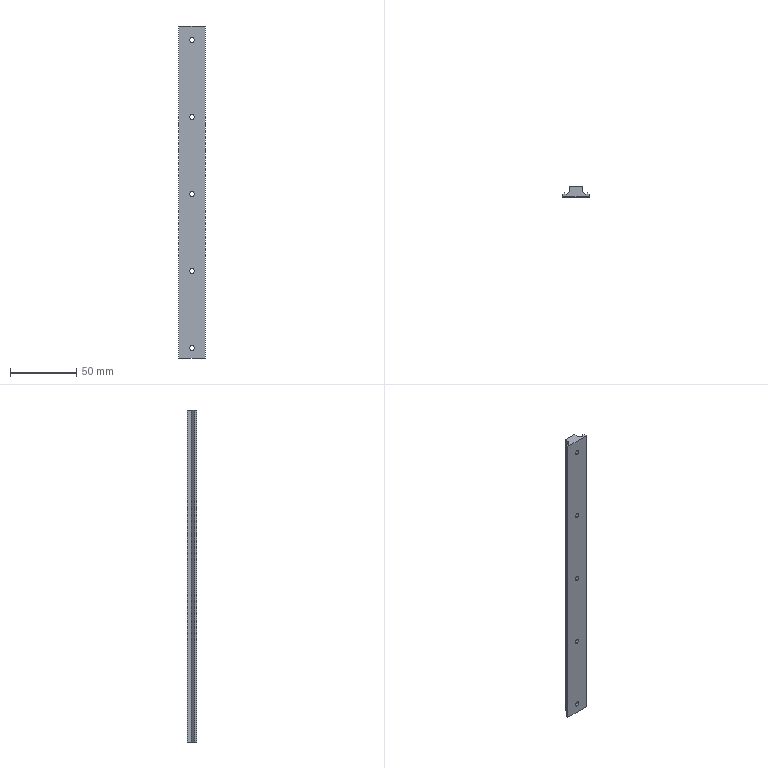Part | STEP file | Guide wheel mechanism revised.sldasm-Part-501 | 1 solid | 41 faces | box 20 x 7.5 x 250 mm | volume 23678 mm3 | plane 21 | cylinder 20 | commonest cylinder face diameters 3.5 x10 6 x10
STEP:
#1=CARTESIAN_POINT('',(0.,0.,237.75));
#2=VERTEX_POINT('',#1);
#3=CARTESIAN_POINT('',(0.,0.,241.25));
#4=VERTEX_POINT('',#3);
#5=CARTESIAN_POINT('',(0.,0.,239.5));
#6=DIRECTION('',(0.,1.,0.));
#7=DIRECTION('',(0.,0.,1.));
#8=AXIS2_PLACEMENT_3D('',#5,#6,#7);
#9=CIRCLE('',#8,1.75);
#10=EDGE_CURVE('',#2,#4,#9,.T.);
#11=ORIENTED_EDGE('',*,*,#10,.F.);
#12=CARTESIAN_POINT('',(0.,3.5,237.75));
#13=VERTEX_POINT('',#12);
#14=CARTESIAN_POINT('',(0.,0.,237.75));
#15=DIRECTION('',(0.,1.,0.));
#16=VECTOR('',#15,1000.);
#17=LINE('',#14,#16);
#18=EDGE_CURVE('',#2,#13,#17,.T.);
#19=ORIENTED_EDGE('',*,*,#18,.T.);
#20=CARTESIAN_POINT('',(0.,3.5,241.25));
#21=VERTEX_POINT('',#20);
#22=CARTESIAN_POINT('',(0.,3.5,239.5));
#23=DIRECTION('',(0.,1.,0.));
#24=DIRECTION('',(0.,0.,1.));
#25=AXIS2_PLACEMENT_3D('',#22,#23,#24);
#26=CIRCLE('',#25,1.75);
#27=EDGE_CURVE('',#13,#21,#26,.T.);
#28=ORIENTED_EDGE('',*,*,#27,.T.);
#29=CARTESIAN_POINT('',(0.,0.,241.25));
#30=DIRECTION('',(0.,1.,0.));
#31=VECTOR('',#30,1000.);
#32=LINE('',#29,#31);
#33=EDGE_CURVE('',#4,#21,#32,.T.);
#34=ORIENTED_EDGE('',*,*,#33,.F.);
#35=EDGE_LOOP('',(#11,#19,#28,#34));
#36=FACE_OUTER_BOUND('',#35,.T.);
#37=CARTESIAN_POINT('',(0.,0.,239.5));
#38=DIRECTION('',(0.,1.,0.));
#39=DIRECTION('',(0.,0.,1.));
#40=AXIS2_PLACEMENT_3D('',#37,#38,#39);
#41=CYLINDRICAL_SURFACE('',#40,1.75);
#42=ADVANCED_FACE('',(#36),#41,.F.);
#43=CARTESIAN_POINT('',(0.,3.5,236.5));
#44=VERTEX_POINT('',#43);
#45=CARTESIAN_POINT('',(0.,3.5,242.5));
#46=VERTEX_POINT('',#45);
#47=CARTESIAN_POINT('',(0.,3.5,239.5));
#48=DIRECTION('',(0.,1.,0.));
#49=DIRECTION('',(0.,0.,1.));
#50=AXIS2_PLACEMENT_3D('',#47,#48,#49);
#51=CIRCLE('',#50,3.);
#52=EDGE_CURVE('',#44,#46,#51,.T.);
#53=ORIENTED_EDGE('',*,*,#52,.F.);
#54=CARTESIAN_POINT('',(0.,7.5,236.5));
#55=VERTEX_POINT('',#54);
#56=CARTESIAN_POINT('',(0.,0.,236.5));
#57=DIRECTION('',(0.,1.,0.));
#58=VECTOR('',#57,1000.);
#59=LINE('',#56,#58);
#60=EDGE_CURVE('',#44,#55,#59,.T.);
#61=ORIENTED_EDGE('',*,*,#60,.T.);
#62=CARTESIAN_POINT('',(0.,7.5,242.5));
#63=VERTEX_POINT('',#62);
#64=CARTESIAN_POINT('',(0.,7.5,239.5));
#65=DIRECTION('',(0.,1.,0.));
#66=DIRECTION('',(0.,0.,1.));
#67=AXIS2_PLACEMENT_3D('',#64,#65,#66);
#68=CIRCLE('',#67,3.);
#69=EDGE_CURVE('',#55,#63,#68,.T.);
#70=ORIENTED_EDGE('',*,*,#69,.T.);
#71=CARTESIAN_POINT('',(0.,0.,242.5));
#72=DIRECTION('',(0.,1.,0.));
#73=VECTOR('',#72,1000.);
#74=LINE('',#71,#73);
#75=EDGE_CURVE('',#46,#63,#74,.T.);
#76=ORIENTED_EDGE('',*,*,#75,.F.);
#77=EDGE_LOOP('',(#53,#61,#70,#76));
#78=FACE_OUTER_BOUND('',#77,.T.);
#79=CARTESIAN_POINT('',(0.,0.,239.5));
#80=DIRECTION('',(0.,1.,0.));
#81=DIRECTION('',(0.,0.,1.));
#82=AXIS2_PLACEMENT_3D('',#79,#80,#81);
#83=CYLINDRICAL_SURFACE('',#82,3.);
#84=ADVANCED_FACE('',(#78),#83,.F.);
#85=CARTESIAN_POINT('',(0.,0.,179.75));
#86=VERTEX_POINT('',#85);
#87=CARTESIAN_POINT('',(0.,0.,183.25));
#88=VERTEX_POINT('',#87);
#89=CARTESIAN_POINT('',(0.,0.,181.5));
#90=DIRECTION('',(0.,1.,0.));
#91=DIRECTION('',(0.,0.,1.));
#92=AXIS2_PLACEMENT_3D('',#89,#90,#91);
#93=CIRCLE('',#92,1.75);
#94=EDGE_CURVE('',#86,#88,#93,.T.);
#95=ORIENTED_EDGE('',*,*,#94,.F.);
#96=CARTESIAN_POINT('',(0.,3.5,179.75));
#97=VERTEX_POINT('',#96);
#98=CARTESIAN_POINT('',(0.,0.,179.75));
#99=DIRECTION('',(0.,1.,0.));
#100=VECTOR('',#99,1000.);
#101=LINE('',#98,#100);
#102=EDGE_CURVE('',#86,#97,#101,.T.);
#103=ORIENTED_EDGE('',*,*,#102,.T.);
#104=CARTESIAN_POINT('',(0.,3.5,183.25));
#105=VERTEX_POINT('',#104);
#106=CARTESIAN_POINT('',(0.,3.5,181.5));
#107=DIRECTION('',(0.,1.,0.));
#108=DIRECTION('',(0.,0.,1.));
#109=AXIS2_PLACEMENT_3D('',#106,#107,#108);
#110=CIRCLE('',#109,1.75);
#111=EDGE_CURVE('',#97,#105,#110,.T.);
#112=ORIENTED_EDGE('',*,*,#111,.T.);
#113=CARTESIAN_POINT('',(0.,0.,183.25));
#114=DIRECTION('',(0.,1.,0.));
#115=VECTOR('',#114,1000.);
#116=LINE('',#113,#115);
#117=EDGE_CURVE('',#88,#105,#116,.T.);
#118=ORIENTED_EDGE('',*,*,#117,.F.);
#119=EDGE_LOOP('',(#95,#103,#112,#118));
#120=FACE_OUTER_BOUND('',#119,.T.);
#121=CARTESIAN_POINT('',(0.,0.,181.5));
#122=DIRECTION('',(0.,1.,0.));
#123=DIRECTION('',(0.,0.,1.));
#124=AXIS2_PLACEMENT_3D('',#121,#122,#123);
#125=CYLINDRICAL_SURFACE('',#124,1.75);
#126=ADVANCED_FACE('',(#120),#125,.F.);
#127=CARTESIAN_POINT('',(0.,3.5,178.5));
#128=VERTEX_POINT('',#127);
#129=CARTESIAN_POINT('',(0.,3.5,184.5));
#130=VERTEX_POINT('',#129);
#131=CARTESIAN_POINT('',(0.,3.5,181.5));
#132=DIRECTION('',(0.,1.,0.));
#133=DIRECTION('',(0.,0.,1.));
#134=AXIS2_PLACEMENT_3D('',#131,#132,#133);
#135=CIRCLE('',#134,3.);
#136=EDGE_CURVE('',#128,#130,#135,.T.);
#137=ORIENTED_EDGE('',*,*,#136,.F.);
#138=CARTESIAN_POINT('',(0.,7.5,178.5));
#139=VERTEX_POINT('',#138);
#140=CARTESIAN_POINT('',(0.,0.,178.5));
#141=DIRECTION('',(0.,1.,0.));
#142=VECTOR('',#141,1000.);
#143=LINE('',#140,#142);
#144=EDGE_CURVE('',#128,#139,#143,.T.);
#145=ORIENTED_EDGE('',*,*,#144,.T.);
#146=CARTESIAN_POINT('',(0.,7.5,184.5));
#147=VERTEX_POINT('',#146);
#148=CARTESIAN_POINT('',(0.,7.5,181.5));
#149=DIRECTION('',(0.,1.,0.));
#150=DIRECTION('',(0.,0.,1.));
#151=AXIS2_PLACEMENT_3D('',#148,#149,#150);
#152=CIRCLE('',#151,3.);
#153=EDGE_CURVE('',#139,#147,#152,.T.);
#154=ORIENTED_EDGE('',*,*,#153,.T.);
#155=CARTESIAN_POINT('',(0.,0.,184.5));
#156=DIRECTION('',(0.,1.,0.));
#157=VECTOR('',#156,1000.);
#158=LINE('',#155,#157);
#159=EDGE_CURVE('',#130,#147,#158,.T.);
#160=ORIENTED_EDGE('',*,*,#159,.F.);
#161=EDGE_LOOP('',(#137,#145,#154,#160));
#162=FACE_OUTER_BOUND('',#161,.T.);
#163=CARTESIAN_POINT('',(0.,0.,181.5));
#164=DIRECTION('',(0.,1.,0.));
#165=DIRECTION('',(0.,0.,1.));
#166=AXIS2_PLACEMENT_3D('',#163,#164,#165);
#167=CYLINDRICAL_SURFACE('',#166,3.);
#168=ADVANCED_FACE('',(#162),#167,.F.);
#169=CARTESIAN_POINT('',(0.,0.,121.75));
#170=VERTEX_POINT('',#169);
#171=CARTESIAN_POINT('',(0.,0.,125.25));
#172=VERTEX_POINT('',#171);
#173=CARTESIAN_POINT('',(0.,0.,123.5));
#174=DIRECTION('',(0.,1.,0.));
#175=DIRECTION('',(0.,0.,1.));
#176=AXIS2_PLACEMENT_3D('',#173,#174,#175);
#177=CIRCLE('',#176,1.75);
#178=EDGE_CURVE('',#170,#172,#177,.T.);
#179=ORIENTED_EDGE('',*,*,#178,.F.);
#180=CARTESIAN_POINT('',(0.,3.5,121.75));
#181=VERTEX_POINT('',#180);
#182=CARTESIAN_POINT('',(0.,0.,121.75));
#183=DIRECTION('',(0.,1.,0.));
#184=VECTOR('',#183,1000.);
#185=LINE('',#182,#184);
#186=EDGE_CURVE('',#170,#181,#185,.T.);
#187=ORIENTED_EDGE('',*,*,#186,.T.);
#188=CARTESIAN_POINT('',(0.,3.5,125.25));
#189=VERTEX_POINT('',#188);
#190=CARTESIAN_POINT('',(0.,3.5,123.5));
#191=DIRECTION('',(0.,1.,0.));
#192=DIRECTION('',(0.,0.,1.));
#193=AXIS2_PLACEMENT_3D('',#190,#191,#192);
#194=CIRCLE('',#193,1.75);
#195=EDGE_CURVE('',#181,#189,#194,.T.);
#196=ORIENTED_EDGE('',*,*,#195,.T.);
#197=CARTESIAN_POINT('',(0.,0.,125.25));
#198=DIRECTION('',(0.,1.,0.));
#199=VECTOR('',#198,1000.);
#200=LINE('',#197,#199);
#201=EDGE_CURVE('',#172,#189,#200,.T.);
#202=ORIENTED_EDGE('',*,*,#201,.F.);
#203=EDGE_LOOP('',(#179,#187,#196,#202));
#204=FACE_OUTER_BOUND('',#203,.T.);
#205=CARTESIAN_POINT('',(0.,0.,123.5));
#206=DIRECTION('',(0.,1.,0.));
#207=DIRECTION('',(0.,0.,1.));
#208=AXIS2_PLACEMENT_3D('',#205,#206,#207);
#209=CYLINDRICAL_SURFACE('',#208,1.75);
#210=ADVANCED_FACE('',(#204),#209,.F.);
#211=CARTESIAN_POINT('',(0.,3.5,120.5));
#212=VERTEX_POINT('',#211);
#213=CARTESIAN_POINT('',(0.,3.5,126.5));
#214=VERTEX_POINT('',#213);
#215=CARTESIAN_POINT('',(0.,3.5,123.5));
#216=DIRECTION('',(0.,1.,0.));
#217=DIRECTION('',(0.,0.,1.));
#218=AXIS2_PLACEMENT_3D('',#215,#216,#217);
#219=CIRCLE('',#218,3.);
#220=EDGE_CURVE('',#212,#214,#219,.T.);
#221=ORIENTED_EDGE('',*,*,#220,.F.);
#222=CARTESIAN_POINT('',(0.,7.5,120.5));
#223=VERTEX_POINT('',#222);
#224=CARTESIAN_POINT('',(0.,0.,120.5));
#225=DIRECTION('',(0.,1.,0.));
#226=VECTOR('',#225,1000.);
#227=LINE('',#224,#226);
#228=EDGE_CURVE('',#212,#223,#227,.T.);
#229=ORIENTED_EDGE('',*,*,#228,.T.);
#230=CARTESIAN_POINT('',(0.,7.5,126.5));
#231=VERTEX_POINT('',#230);
#232=CARTESIAN_POINT('',(0.,7.5,123.5));
#233=DIRECTION('',(0.,1.,0.));
#234=DIRECTION('',(0.,0.,1.));
#235=AXIS2_PLACEMENT_3D('',#232,#233,#234);
#236=CIRCLE('',#235,3.);
#237=EDGE_CURVE('',#223,#231,#236,.T.);
#238=ORIENTED_EDGE('',*,*,#237,.T.);
#239=CARTESIAN_POINT('',(0.,0.,126.5));
#240=DIRECTION('',(0.,1.,0.));
#241=VECTOR('',#240,1000.);
#242=LINE('',#239,#241);
#243=EDGE_CURVE('',#214,#231,#242,.T.);
#244=ORIENTED_EDGE('',*,*,#243,.F.);
#245=EDGE_LOOP('',(#221,#229,#238,#244));
#246=FACE_OUTER_BOUND('',#245,.T.);
#247=CARTESIAN_POINT('',(0.,0.,123.5));
#248=DIRECTION('',(0.,1.,0.));
#249=DIRECTION('',(0.,0.,1.));
#250=AXIS2_PLACEMENT_3D('',#247,#248,#249);
#251=CYLINDRICAL_SURFACE('',#250,3.);
#252=ADVANCED_FACE('',(#246),#251,.F.);
#253=CARTESIAN_POINT('',(0.,0.,63.75));
#254=VERTEX_POINT('',#253);
#255=CARTESIAN_POINT('',(0.,0.,67.25));
#256=VERTEX_POINT('',#255);
#257=CARTESIAN_POINT('',(0.,0.,65.5));
#258=DIRECTION('',(0.,1.,0.));
#259=DIRECTION('',(0.,0.,1.));
#260=AXIS2_PLACEMENT_3D('',#257,#258,#259);
#261=CIRCLE('',#260,1.75);
#262=EDGE_CURVE('',#254,#256,#261,.T.);
#263=ORIENTED_EDGE('',*,*,#262,.F.);
#264=CARTESIAN_POINT('',(0.,3.5,63.75));
#265=VERTEX_POINT('',#264);
#266=CARTESIAN_POINT('',(0.,0.,63.75));
#267=DIRECTION('',(0.,1.,0.));
#268=VECTOR('',#267,1000.);
#269=LINE('',#266,#268);
#270=EDGE_CURVE('',#254,#265,#269,.T.);
#271=ORIENTED_EDGE('',*,*,#270,.T.);
#272=CARTESIAN_POINT('',(0.,3.5,67.25));
#273=VERTEX_POINT('',#272);
#274=CARTESIAN_POINT('',(0.,3.5,65.5));
#275=DIRECTION('',(0.,1.,0.));
#276=DIRECTION('',(0.,0.,1.));
#277=AXIS2_PLACEMENT_3D('',#274,#275,#276);
#278=CIRCLE('',#277,1.75);
#279=EDGE_CURVE('',#265,#273,#278,.T.);
#280=ORIENTED_EDGE('',*,*,#279,.T.);
#281=CARTESIAN_POINT('',(0.,0.,67.25));
#282=DIRECTION('',(0.,1.,0.));
#283=VECTOR('',#282,1000.);
#284=LINE('',#281,#283);
#285=EDGE_CURVE('',#256,#273,#284,.T.);
#286=ORIENTED_EDGE('',*,*,#285,.F.);
#287=EDGE_LOOP('',(#263,#271,#280,#286));
#288=FACE_OUTER_BOUND('',#287,.T.);
#289=CARTESIAN_POINT('',(0.,0.,65.5));
#290=DIRECTION('',(0.,1.,0.));
#291=DIRECTION('',(0.,0.,1.));
#292=AXIS2_PLACEMENT_3D('',#289,#290,#291);
#293=CYLINDRICAL_SURFACE('',#292,1.75);
#294=ADVANCED_FACE('',(#288),#293,.F.);
#295=CARTESIAN_POINT('',(0.,3.5,62.5));
#296=VERTEX_POINT('',#295);
#297=CARTESIAN_POINT('',(0.,3.5,68.5));
#298=VERTEX_POINT('',#297);
#299=CARTESIAN_POINT('',(0.,3.5,65.5));
#300=DIRECTION('',(0.,1.,0.));
#301=DIRECTION('',(0.,0.,1.));
#302=AXIS2_PLACEMENT_3D('',#299,#300,#301);
#303=CIRCLE('',#302,3.);
#304=EDGE_CURVE('',#296,#298,#303,.T.);
#305=ORIENTED_EDGE('',*,*,#304,.F.);
#306=CARTESIAN_POINT('',(0.,7.5,62.5));
#307=VERTEX_POINT('',#306);
#308=CARTESIAN_POINT('',(0.,0.,62.5));
#309=DIRECTION('',(0.,1.,0.));
#310=VECTOR('',#309,1000.);
#311=LINE('',#308,#310);
#312=EDGE_CURVE('',#296,#307,#311,.T.);
#313=ORIENTED_EDGE('',*,*,#312,.T.);
#314=CARTESIAN_POINT('',(0.,7.5,68.5));
#315=VERTEX_POINT('',#314);
#316=CARTESIAN_POINT('',(0.,7.5,65.5));
#317=DIRECTION('',(0.,1.,0.));
#318=DIRECTION('',(0.,0.,1.));
#319=AXIS2_PLACEMENT_3D('',#316,#317,#318);
#320=CIRCLE('',#319,3.);
#321=EDGE_CURVE('',#307,#315,#320,.T.);
#322=ORIENTED_EDGE('',*,*,#321,.T.);
#323=CARTESIAN_POINT('',(0.,0.,68.5));
#324=DIRECTION('',(0.,1.,0.));
#325=VECTOR('',#324,1000.);
#326=LINE('',#323,#325);
#327=EDGE_CURVE('',#298,#315,#326,.T.);
#328=ORIENTED_EDGE('',*,*,#327,.F.);
#329=EDGE_LOOP('',(#305,#313,#322,#328));
#330=FACE_OUTER_BOUND('',#329,.T.);
#331=CARTESIAN_POINT('',(0.,0.,65.5));
#332=DIRECTION('',(0.,1.,0.));
#333=DIRECTION('',(0.,0.,1.));
#334=AXIS2_PLACEMENT_3D('',#331,#332,#333);
#335=CYLINDRICAL_SURFACE('',#334,3.);
#336=ADVANCED_FACE('',(#330),#335,.F.);
#337=CARTESIAN_POINT('',(0.,0.,5.75));
#338=VERTEX_POINT('',#337);
#339=CARTESIAN_POINT('',(0.,0.,9.25));
#340=VERTEX_POINT('',#339);
#341=CARTESIAN_POINT('',(0.,0.,7.5));
#342=DIRECTION('',(0.,1.,0.));
#343=DIRECTION('',(0.,0.,1.));
#344=AXIS2_PLACEMENT_3D('',#341,#342,#343);
#345=CIRCLE('',#344,1.75);
#346=EDGE_CURVE('',#338,#340,#345,.T.);
#347=ORIENTED_EDGE('',*,*,#346,.F.);
#348=CARTESIAN_POINT('',(0.,3.5,5.75));
#349=VERTEX_POINT('',#348);
#350=CARTESIAN_POINT('',(0.,0.,5.75));
#351=DIRECTION('',(0.,1.,0.));
#352=VECTOR('',#351,1000.);
#353=LINE('',#350,#352);
#354=EDGE_CURVE('',#338,#349,#353,.T.);
#355=ORIENTED_EDGE('',*,*,#354,.T.);
#356=CARTESIAN_POINT('',(0.,3.5,9.25));
#357=VERTEX_POINT('',#356);
#358=CARTESIAN_POINT('',(0.,3.5,7.5));
#359=DIRECTION('',(0.,1.,0.));
#360=DIRECTION('',(0.,0.,1.));
#361=AXIS2_PLACEMENT_3D('',#358,#359,#360);
#362=CIRCLE('',#361,1.75);
#363=EDGE_CURVE('',#349,#357,#362,.T.);
#364=ORIENTED_EDGE('',*,*,#363,.T.);
#365=CARTESIAN_POINT('',(0.,0.,9.25));
#366=DIRECTION('',(0.,1.,0.));
#367=VECTOR('',#366,1000.);
#368=LINE('',#365,#367);
#369=EDGE_CURVE('',#340,#357,#368,.T.);
#370=ORIENTED_EDGE('',*,*,#369,.F.);
#371=EDGE_LOOP('',(#347,#355,#364,#370));
#372=FACE_OUTER_BOUND('',#371,.T.);
#373=CARTESIAN_POINT('',(0.,0.,7.5));
#374=DIRECTION('',(0.,1.,0.));
#375=DIRECTION('',(0.,0.,1.));
#376=AXIS2_PLACEMENT_3D('',#373,#374,#375);
#377=CYLINDRICAL_SURFACE('',#376,1.75);
#378=ADVANCED_FACE('',(#372),#377,.F.);
#379=CARTESIAN_POINT('',(0.,3.5,4.5));
#380=VERTEX_POINT('',#379);
#381=CARTESIAN_POINT('',(0.,3.5,10.5));
#382=VERTEX_POINT('',#381);
#383=CARTESIAN_POINT('',(0.,3.5,7.5));
#384=DIRECTION('',(0.,1.,0.));
#385=DIRECTION('',(0.,0.,1.));
#386=AXIS2_PLACEMENT_3D('',#383,#384,#385);
#387=CIRCLE('',#386,3.);
#388=EDGE_CURVE('',#380,#382,#387,.T.);
#389=ORIENTED_EDGE('',*,*,#388,.F.);
#390=CARTESIAN_POINT('',(0.,7.5,4.5));
#391=VERTEX_POINT('',#390);
#392=CARTESIAN_POINT('',(0.,0.,4.5));
#393=DIRECTION('',(0.,1.,0.));
#394=VECTOR('',#393,1000.);
#395=LINE('',#392,#394);
#396=EDGE_CURVE('',#380,#391,#395,.T.);
#397=ORIENTED_EDGE('',*,*,#396,.T.);
#398=CARTESIAN_POINT('',(0.,7.5,10.5));
#399=VERTEX_POINT('',#398);
#400=CARTESIAN_POINT('',(0.,7.5,7.5));
#401=DIRECTION('',(0.,1.,0.));
#402=DIRECTION('',(0.,0.,1.));
#403=AXIS2_PLACEMENT_3D('',#400,#401,#402);
#404=CIRCLE('',#403,3.);
#405=EDGE_CURVE('',#391,#399,#404,.T.);
#406=ORIENTED_EDGE('',*,*,#405,.T.);
#407=CARTESIAN_POINT('',(0.,0.,10.5));
#408=DIRECTION('',(0.,1.,0.));
#409=VECTOR('',#408,1000.);
#410=LINE('',#407,#409);
#411=EDGE_CURVE('',#382,#399,#410,.T.);
#412=ORIENTED_EDGE('',*,*,#411,.F.);
#413=EDGE_LOOP('',(#389,#397,#406,#412));
#414=FACE_OUTER_BOUND('',#413,.T.);
#415=CARTESIAN_POINT('',(0.,0.,7.5));
#416=DIRECTION('',(0.,1.,0.));
#417=DIRECTION('',(0.,0.,1.));
#418=AXIS2_PLACEMENT_3D('',#415,#416,#417);
#419=CYLINDRICAL_SURFACE('',#418,3.);
#420=ADVANCED_FACE('',(#414),#419,.F.);
#421=CARTESIAN_POINT('',(0.,0.,181.5));
#422=DIRECTION('',(0.,1.,0.));
#423=DIRECTION('',(0.,0.,1.));
#424=AXIS2_PLACEMENT_3D('',#421,#422,#423);
#425=CIRCLE('',#424,1.75);
#426=EDGE_CURVE('',#88,#86,#425,.T.);
#427=ORIENTED_EDGE('',*,*,#426,.T.);
#428=ORIENTED_EDGE('',*,*,#94,.T.);
#429=EDGE_LOOP('',(#427,#428));
#430=FACE_BOUND('',#429,.T.);
#431=CARTESIAN_POINT('',(0.,0.,65.5));
#432=DIRECTION('',(0.,1.,0.));
#433=DIRECTION('',(0.,0.,1.));
#434=AXIS2_PLACEMENT_3D('',#431,#432,#433);
#435=CIRCLE('',#434,1.75);
#436=EDGE_CURVE('',#256,#254,#435,.T.);
#437=ORIENTED_EDGE('',*,*,#436,.T.);
#438=ORIENTED_EDGE('',*,*,#262,.T.);
#439=EDGE_LOOP('',(#437,#438));
#440=FACE_BOUND('',#439,.T.);
#441=CARTESIAN_POINT('',(-10.,0.,0.));
#442=VERTEX_POINT('',#441);
#443=CARTESIAN_POINT('',(10.,0.,0.));
#444=VERTEX_POINT('',#443);
#445=CARTESIAN_POINT('',(-10.,0.,0.));
#446=DIRECTION('',(1.,0.,0.));
#447=VECTOR('',#446,1000.);
#448=LINE('',#445,#447);
#449=EDGE_CURVE('',#442,#444,#448,.T.);
#450=ORIENTED_EDGE('',*,*,#449,.T.);
#451=CARTESIAN_POINT('',(10.,0.,250.));
#452=VERTEX_POINT('',#451);
#453=CARTESIAN_POINT('',(10.,0.,250.));
#454=DIRECTION('',(0.,0.,-1.));
#455=VECTOR('',#454,1000.);
#456=LINE('',#453,#455);
#457=EDGE_CURVE('',#452,#444,#456,.T.);
#458=ORIENTED_EDGE('',*,*,#457,.F.);
#459=CARTESIAN_POINT('',(-10.,0.,250.));
#460=VERTEX_POINT('',#459);
#461=CARTESIAN_POINT('',(-10.,0.,250.));
#462=DIRECTION('',(1.,0.,0.));
#463=VECTOR('',#462,1000.);
#464=LINE('',#461,#463);
#465=EDGE_CURVE('',#460,#452,#464,.T.);
#466=ORIENTED_EDGE('',*,*,#465,.F.);
#467=CARTESIAN_POINT('',(-10.,0.,250.));
#468=DIRECTION('',(0.,0.,-1.));
#469=VECTOR('',#468,1000.);
#470=LINE('',#467,#469);
#471=EDGE_CURVE('',#460,#442,#470,.T.);
#472=ORIENTED_EDGE('',*,*,#471,.T.);
#473=EDGE_LOOP('',(#450,#458,#466,#472));
#474=FACE_OUTER_BOUND('',#473,.T.);
#475=CARTESIAN_POINT('',(0.,0.,7.5));
#476=DIRECTION('',(0.,1.,0.));
#477=DIRECTION('',(0.,0.,1.));
#478=AXIS2_PLACEMENT_3D('',#475,#476,#477);
#479=CIRCLE('',#478,1.75);
#480=EDGE_CURVE('',#340,#338,#479,.T.);
#481=ORIENTED_EDGE('',*,*,#480,.T.);
#482=ORIENTED_EDGE('',*,*,#346,.T.);
#483=EDGE_LOOP('',(#481,#482));
#484=FACE_BOUND('',#483,.T.);
#485=CARTESIAN_POINT('',(0.,0.,123.5));
#486=DIRECTION('',(0.,1.,0.));
#487=DIRECTION('',(0.,0.,1.));
#488=AXIS2_PLACEMENT_3D('',#485,#486,#487);
#489=CIRCLE('',#488,1.75);
#490=EDGE_CURVE('',#172,#170,#489,.T.);
#491=ORIENTED_EDGE('',*,*,#490,.T.);
#492=ORIENTED_EDGE('',*,*,#178,.T.);
#493=EDGE_LOOP('',(#491,#492));
#494=FACE_BOUND('',#493,.T.);
#495=CARTESIAN_POINT('',(0.,0.,239.5));
#496=DIRECTION('',(0.,1.,0.));
#497=DIRECTION('',(0.,0.,1.));
#498=AXIS2_PLACEMENT_3D('',#495,#496,#497);
#499=CIRCLE('',#498,1.75);
#500=EDGE_CURVE('',#4,#2,#499,.T.);
#501=ORIENTED_EDGE('',*,*,#500,.T.);
#502=ORIENTED_EDGE('',*,*,#10,.T.);
#503=EDGE_LOOP('',(#501,#502));
#504=FACE_BOUND('',#503,.T.);
#505=CARTESIAN_POINT('',(-10.,0.,250.));
#506=DIRECTION('',(0.,1.,0.));
#507=DIRECTION('',(0.,0.,1.));
#508=AXIS2_PLACEMENT_3D('',#505,#506,#507);
#509=PLANE('',#508);
#510=ADVANCED_FACE('',(#430,#440,#474,#484,#494,#504),#509,.F.);
#511=CARTESIAN_POINT('',(0.,7.5,181.5));
#512=DIRECTION('',(0.,1.,0.));
#513=DIRECTION('',(0.,0.,1.));
#514=AXIS2_PLACEMENT_3D('',#511,#512,#513);
#515=CIRCLE('',#514,3.);
#516=EDGE_CURVE('',#147,#139,#515,.T.);
#517=ORIENTED_EDGE('',*,*,#516,.F.);
#518=ORIENTED_EDGE('',*,*,#153,.F.);
#519=EDGE_LOOP('',(#517,#518));
#520=FACE_BOUND('',#519,.T.);
#521=CARTESIAN_POINT('',(0.,7.5,65.5));
#522=DIRECTION('',(0.,1.,0.));
#523=DIRECTION('',(0.,0.,1.));
#524=AXIS2_PLACEMENT_3D('',#521,#522,#523);
#525=CIRCLE('',#524,3.);
#526=EDGE_CURVE('',#315,#307,#525,.T.);
#527=ORIENTED_EDGE('',*,*,#526,.F.);
#528=ORIENTED_EDGE('',*,*,#321,.F.);
#529=EDGE_LOOP('',(#527,#528));
#530=FACE_BOUND('',#529,.T.);
#531=CARTESIAN_POINT('',(4.864,7.5,0.));
#532=VERTEX_POINT('',#531);
#533=CARTESIAN_POINT('',(-4.864,7.5,0.));
#534=VERTEX_POINT('',#533);
#535=CARTESIAN_POINT('',(4.864,7.5,0.));
#536=DIRECTION('',(-1.,0.,0.));
#537=VECTOR('',#536,1000.);
#538=LINE('',#535,#537);
#539=EDGE_CURVE('',#532,#534,#538,.T.);
#540=ORIENTED_EDGE('',*,*,#539,.T.);
#541=CARTESIAN_POINT('',(-4.864,7.5,250.));
#542=VERTEX_POINT('',#541);
#543=CARTESIAN_POINT('',(-4.864,7.5,250.));
#544=DIRECTION('',(0.,0.,-1.));
#545=VECTOR('',#544,1000.);
#546=LINE('',#543,#545);
#547=EDGE_CURVE('',#542,#534,#546,.T.);
#548=ORIENTED_EDGE('',*,*,#547,.F.);
#549=CARTESIAN_POINT('',(4.864,7.5,250.));
#550=VERTEX_POINT('',#549);
#551=CARTESIAN_POINT('',(4.864,7.5,250.));
#552=DIRECTION('',(-1.,0.,0.));
#553=VECTOR('',#552,1000.);
#554=LINE('',#551,#553);
#555=EDGE_CURVE('',#550,#542,#554,.T.);
#556=ORIENTED_EDGE('',*,*,#555,.F.);
#557=CARTESIAN_POINT('',(4.864,7.5,250.));
#558=DIRECTION('',(0.,0.,-1.));
#559=VECTOR('',#558,1000.);
#560=LINE('',#557,#559);
#561=EDGE_CURVE('',#550,#532,#560,.T.);
#562=ORIENTED_EDGE('',*,*,#561,.T.);
#563=EDGE_LOOP('',(#540,#548,#556,#562));
#564=FACE_OUTER_BOUND('',#563,.T.);
#565=CARTESIAN_POINT('',(0.,7.5,7.5));
#566=DIRECTION('',(0.,1.,0.));
#567=DIRECTION('',(0.,0.,1.));
#568=AXIS2_PLACEMENT_3D('',#565,#566,#567);
#569=CIRCLE('',#568,3.);
#570=EDGE_CURVE('',#399,#391,#569,.T.);
#571=ORIENTED_EDGE('',*,*,#570,.F.);
#572=ORIENTED_EDGE('',*,*,#405,.F.);
#573=EDGE_LOOP('',(#571,#572));
#574=FACE_BOUND('',#573,.T.);
#575=CARTESIAN_POINT('',(0.,7.5,123.5));
#576=DIRECTION('',(0.,1.,0.));
#577=DIRECTION('',(0.,0.,1.));
#578=AXIS2_PLACEMENT_3D('',#575,#576,#577);
#579=CIRCLE('',#578,3.);
#580=EDGE_CURVE('',#231,#223,#579,.T.);
#581=ORIENTED_EDGE('',*,*,#580,.F.);
#582=ORIENTED_EDGE('',*,*,#237,.F.);
#583=EDGE_LOOP('',(#581,#582));
#584=FACE_BOUND('',#583,.T.);
#585=CARTESIAN_POINT('',(0.,7.5,239.5));
#586=DIRECTION('',(0.,1.,0.));
#587=DIRECTION('',(0.,0.,1.));
#588=AXIS2_PLACEMENT_3D('',#585,#586,#587);
#589=CIRCLE('',#588,3.);
#590=EDGE_CURVE('',#63,#55,#589,.T.);
#591=ORIENTED_EDGE('',*,*,#590,.F.);
#592=ORIENTED_EDGE('',*,*,#69,.F.);
#593=EDGE_LOOP('',(#591,#592));
#594=FACE_BOUND('',#593,.T.);
#595=CARTESIAN_POINT('',(4.864,7.5,250.));
#596=DIRECTION('',(0.,-1.,0.));
#597=DIRECTION('',(0.,0.,-1.));
#598=AXIS2_PLACEMENT_3D('',#595,#596,#597);
#599=PLANE('',#598);
#600=ADVANCED_FACE('',(#520,#530,#564,#574,#584,#594),#599,.F.);
#601=CARTESIAN_POINT('',(-10.,1.8,0.));
#602=VERTEX_POINT('',#601);
#603=CARTESIAN_POINT('',(-10.,1.8,0.));
#604=DIRECTION('',(0.,-1.,0.));
#605=VECTOR('',#604,1000.);
#606=LINE('',#603,#605);
#607=EDGE_CURVE('',#602,#442,#606,.T.);
#608=ORIENTED_EDGE('',*,*,#607,.T.);
#609=ORIENTED_EDGE('',*,*,#471,.F.);
#610=CARTESIAN_POINT('',(-10.,1.8,250.));
#611=VERTEX_POINT('',#610);
#612=CARTESIAN_POINT('',(-10.,1.8,250.));
#613=DIRECTION('',(0.,-1.,0.));
#614=VECTOR('',#613,1000.);
#615=LINE('',#612,#614);
#616=EDGE_CURVE('',#611,#460,#615,.T.);
#617=ORIENTED_EDGE('',*,*,#616,.F.);
#618=CARTESIAN_POINT('',(-10.,1.8,250.));
#619=DIRECTION('',(0.,0.,-1.));
#620=VECTOR('',#619,1000.);
#621=LINE('',#618,#620);
#622=EDGE_CURVE('',#611,#602,#621,.T.);
#623=ORIENTED_EDGE('',*,*,#622,.T.);
#624=EDGE_LOOP('',(#608,#609,#617,#623));
#625=FACE_OUTER_BOUND('',#624,.T.);
#626=CARTESIAN_POINT('',(-10.,1.8,250.));
#627=DIRECTION('',(1.,0.,0.));
#628=DIRECTION('',(0.,0.,-1.));
#629=AXIS2_PLACEMENT_3D('',#626,#627,#628);
#630=PLANE('',#629);
#631=ADVANCED_FACE('',(#625),#630,.F.);
#632=CARTESIAN_POINT('',(10.,1.8,0.));
#633=VERTEX_POINT('',#632);
#634=CARTESIAN_POINT('',(10.,0.,0.));
#635=DIRECTION('',(0.,1.,0.));
#636=VECTOR('',#635,1000.);
#637=LINE('',#634,#636);
#638=EDGE_CURVE('',#444,#633,#637,.T.);
#639=ORIENTED_EDGE('',*,*,#638,.T.);
#640=CARTESIAN_POINT('',(10.,1.8,250.));
#641=VERTEX_POINT('',#640);
#642=CARTESIAN_POINT('',(10.,1.8,250.));
#643=DIRECTION('',(0.,0.,-1.));
#644=VECTOR('',#643,1000.);
#645=LINE('',#642,#644);
#646=EDGE_CURVE('',#641,#633,#645,.T.);
#647=ORIENTED_EDGE('',*,*,#646,.F.);
#648=CARTESIAN_POINT('',(10.,0.,250.));
#649=DIRECTION('',(0.,1.,0.));
#650=VECTOR('',#649,1000.);
#651=LINE('',#648,#650);
#652=EDGE_CURVE('',#452,#641,#651,.T.);
#653=ORIENTED_EDGE('',*,*,#652,.F.);
#654=ORIENTED_EDGE('',*,*,#457,.T.);
#655=EDGE_LOOP('',(#639,#647,#653,#654));
#656=FACE_OUTER_BOUND('',#655,.T.);
#657=CARTESIAN_POINT('',(10.,0.,250.));
#658=DIRECTION('',(-1.,0.,0.));
#659=DIRECTION('',(0.,0.,1.));
#660=AXIS2_PLACEMENT_3D('',#657,#658,#659);
#661=PLANE('',#660);
#662=ADVANCED_FACE('',(#656),#661,.F.);
#663=CARTESIAN_POINT('',(8.993,2.807,0.));
#664=VERTEX_POINT('',#663);
#665=CARTESIAN_POINT('',(10.,1.8,0.));
#666=DIRECTION('',(-0.7071,0.7071,0.));
#667=VECTOR('',#666,1000.);
#668=LINE('',#665,#667);
#669=EDGE_CURVE('',#633,#664,#668,.T.);
#670=ORIENTED_EDGE('',*,*,#669,.T.);
#671=CARTESIAN_POINT('',(8.993,2.807,250.));
#672=VERTEX_POINT('',#671);
#673=CARTESIAN_POINT('',(8.993,2.807,250.));
#674=DIRECTION('',(0.,0.,-1.));
#675=VECTOR('',#674,1000.);
#676=LINE('',#673,#675);
#677=EDGE_CURVE('',#672,#664,#676,.T.);
#678=ORIENTED_EDGE('',*,*,#677,.F.);
#679=CARTESIAN_POINT('',(10.,1.8,250.));
#680=DIRECTION('',(-0.7071,0.7071,0.));
#681=VECTOR('',#680,1000.);
#682=LINE('',#679,#681);
#683=EDGE_CURVE('',#641,#672,#682,.T.);
#684=ORIENTED_EDGE('',*,*,#683,.F.);
#685=ORIENTED_EDGE('',*,*,#646,.T.);
#686=EDGE_LOOP('',(#670,#678,#684,#685));
#687=FACE_OUTER_BOUND('',#686,.T.);
#688=CARTESIAN_POINT('',(10.,1.8,250.));
#689=DIRECTION('',(-0.7071,-0.7071,0.));
#690=DIRECTION('',(0.7071,-0.7071,0.));
#691=AXIS2_PLACEMENT_3D('',#688,#689,#690);
#692=PLANE('',#691);
#693=ADVANCED_FACE('',(#687),#692,.F.);
#694=CARTESIAN_POINT('',(7.508,1.322,0.));
#695=VERTEX_POINT('',#694);
#696=CARTESIAN_POINT('',(8.993,2.807,0.));
#697=DIRECTION('',(-0.7071,-0.7071,0.));
#698=VECTOR('',#697,1000.);
#699=LINE('',#696,#698);
#700=EDGE_CURVE('',#664,#695,#699,.T.);
#701=ORIENTED_EDGE('',*,*,#700,.T.);
#702=CARTESIAN_POINT('',(7.508,1.322,250.));
#703=VERTEX_POINT('',#702);
#704=CARTESIAN_POINT('',(7.508,1.322,250.));
#705=DIRECTION('',(0.,0.,-1.));
#706=VECTOR('',#705,1000.);
#707=LINE('',#704,#706);
#708=EDGE_CURVE('',#703,#695,#707,.T.);
#709=ORIENTED_EDGE('',*,*,#708,.F.);
#710=CARTESIAN_POINT('',(8.993,2.807,250.));
#711=DIRECTION('',(-0.7071,-0.7071,0.));
#712=VECTOR('',#711,1000.);
#713=LINE('',#710,#712);
#714=EDGE_CURVE('',#672,#703,#713,.T.);
#715=ORIENTED_EDGE('',*,*,#714,.F.);
#716=ORIENTED_EDGE('',*,*,#677,.T.);
#717=EDGE_LOOP('',(#701,#709,#715,#716));
#718=FACE_OUTER_BOUND('',#717,.T.);
#719=CARTESIAN_POINT('',(8.993,2.807,250.));
#720=DIRECTION('',(0.7071,-0.7071,0.));
#721=DIRECTION('',(0.7071,0.7071,0.));
#722=AXIS2_PLACEMENT_3D('',#719,#720,#721);
#723=PLANE('',#722);
#724=ADVANCED_FACE('',(#718),#723,.F.);
#725=CARTESIAN_POINT('',(4.68,4.151,0.));
#726=VERTEX_POINT('',#725);
#727=CARTESIAN_POINT('',(7.508,1.322,0.));
#728=DIRECTION('',(-0.7071,0.7071,0.));
#729=VECTOR('',#728,1000.);
#730=LINE('',#727,#729);
#731=EDGE_CURVE('',#695,#726,#730,.T.);
#732=ORIENTED_EDGE('',*,*,#731,.T.);
#733=CARTESIAN_POINT('',(4.68,4.151,250.));
#734=VERTEX_POINT('',#733);
#735=CARTESIAN_POINT('',(4.68,4.151,250.));
#736=DIRECTION('',(0.,0.,-1.));
#737=VECTOR('',#736,1000.);
#738=LINE('',#735,#737);
#739=EDGE_CURVE('',#734,#726,#738,.T.);
#740=ORIENTED_EDGE('',*,*,#739,.F.);
#741=CARTESIAN_POINT('',(7.508,1.322,250.));
#742=DIRECTION('',(-0.7071,0.7071,0.));
#743=VECTOR('',#742,1000.);
#744=LINE('',#741,#743);
#745=EDGE_CURVE('',#703,#734,#744,.T.);
#746=ORIENTED_EDGE('',*,*,#745,.F.);
#747=ORIENTED_EDGE('',*,*,#708,.T.);
#748=EDGE_LOOP('',(#732,#740,#746,#747));
#749=FACE_OUTER_BOUND('',#748,.T.);
#750=CARTESIAN_POINT('',(7.508,1.322,250.));
#751=DIRECTION('',(-0.7071,-0.7071,0.));
#752=DIRECTION('',(0.7071,-0.7071,0.));
#753=AXIS2_PLACEMENT_3D('',#750,#751,#752);
#754=PLANE('',#753);
#755=ADVANCED_FACE('',(#749),#754,.F.);
#756=CARTESIAN_POINT('',(4.864,4.336,0.));
#757=VERTEX_POINT('',#756);
#758=CARTESIAN_POINT('',(4.68,4.151,0.));
#759=DIRECTION('',(0.7071,0.7071,0.));
#760=VECTOR('',#759,1000.);
#761=LINE('',#758,#760);
#762=EDGE_CURVE('',#726,#757,#761,.T.);
#763=ORIENTED_EDGE('',*,*,#762,.T.);
#764=CARTESIAN_POINT('',(4.864,4.336,250.));
#765=VERTEX_POINT('',#764);
#766=CARTESIAN_POINT('',(4.864,4.336,250.));
#767=DIRECTION('',(0.,0.,-1.));
#768=VECTOR('',#767,1000.);
#769=LINE('',#766,#768);
#770=EDGE_CURVE('',#765,#757,#769,.T.);
#771=ORIENTED_EDGE('',*,*,#770,.F.);
#772=CARTESIAN_POINT('',(4.68,4.151,250.));
#773=DIRECTION('',(0.7071,0.7071,0.));
#774=VECTOR('',#773,1000.);
#775=LINE('',#772,#774);
#776=EDGE_CURVE('',#734,#765,#775,.T.);
#777=ORIENTED_EDGE('',*,*,#776,.F.);
#778=ORIENTED_EDGE('',*,*,#739,.T.);
#779=EDGE_LOOP('',(#763,#771,#777,#778));
#780=FACE_OUTER_BOUND('',#779,.T.);
#781=CARTESIAN_POINT('',(4.68,4.151,250.));
#782=DIRECTION('',(-0.7071,0.7071,0.));
#783=DIRECTION('',(-0.7071,-0.7071,0.));
#784=AXIS2_PLACEMENT_3D('',#781,#782,#783);
#785=PLANE('',#784);
#786=ADVANCED_FACE('',(#780),#785,.F.);
#787=CARTESIAN_POINT('',(4.864,4.336,0.));
#788=DIRECTION('',(0.,1.,0.));
#789=VECTOR('',#788,1000.);
#790=LINE('',#787,#789);
#791=EDGE_CURVE('',#757,#532,#790,.T.);
#792=ORIENTED_EDGE('',*,*,#791,.T.);
#793=ORIENTED_EDGE('',*,*,#561,.F.);
#794=CARTESIAN_POINT('',(4.864,4.336,250.));
#795=DIRECTION('',(0.,1.,0.));
#796=VECTOR('',#795,1000.);
#797=LINE('',#794,#796);
#798=EDGE_CURVE('',#765,#550,#797,.T.);
#799=ORIENTED_EDGE('',*,*,#798,.F.);
#800=ORIENTED_EDGE('',*,*,#770,.T.);
#801=EDGE_LOOP('',(#792,#793,#799,#800));
#802=FACE_OUTER_BOUND('',#801,.T.);
#803=CARTESIAN_POINT('',(4.864,4.336,250.));
#804=DIRECTION('',(-1.,0.,0.));
#805=DIRECTION('',(0.,0.,1.));
#806=AXIS2_PLACEMENT_3D('',#803,#804,#805);
#807=PLANE('',#806);
#808=ADVANCED_FACE('',(#802),#807,.F.);
#809=CARTESIAN_POINT('',(-4.864,4.336,0.));
#810=VERTEX_POINT('',#809);
#811=CARTESIAN_POINT('',(-4.864,7.5,0.));
#812=DIRECTION('',(0.,-1.,0.));
#813=VECTOR('',#812,1000.);
#814=LINE('',#811,#813);
#815=EDGE_CURVE('',#534,#810,#814,.T.);
#816=ORIENTED_EDGE('',*,*,#815,.T.);
#817=CARTESIAN_POINT('',(-4.864,4.336,250.));
#818=VERTEX_POINT('',#817);
#819=CARTESIAN_POINT('',(-4.864,4.336,250.));
#820=DIRECTION('',(0.,0.,-1.));
#821=VECTOR('',#820,1000.);
#822=LINE('',#819,#821);
#823=EDGE_CURVE('',#818,#810,#822,.T.);
#824=ORIENTED_EDGE('',*,*,#823,.F.);
#825=CARTESIAN_POINT('',(-4.864,7.5,250.));
#826=DIRECTION('',(0.,-1.,0.));
#827=VECTOR('',#826,1000.);
#828=LINE('',#825,#827);
#829=EDGE_CURVE('',#542,#818,#828,.T.);
#830=ORIENTED_EDGE('',*,*,#829,.F.);
#831=ORIENTED_EDGE('',*,*,#547,.T.);
#832=EDGE_LOOP('',(#816,#824,#830,#831));
#833=FACE_OUTER_BOUND('',#832,.T.);
#834=CARTESIAN_POINT('',(-4.864,7.5,250.));
#835=DIRECTION('',(1.,0.,0.));
#836=DIRECTION('',(0.,0.,-1.));
#837=AXIS2_PLACEMENT_3D('',#834,#835,#836);
#838=PLANE('',#837);
#839=ADVANCED_FACE('',(#833),#838,.F.);
#840=CARTESIAN_POINT('',(-4.68,4.151,0.));
#841=VERTEX_POINT('',#840);
#842=CARTESIAN_POINT('',(-4.864,4.336,0.));
#843=DIRECTION('',(0.7071,-0.7071,0.));
#844=VECTOR('',#843,1000.);
#845=LINE('',#842,#844);
#846=EDGE_CURVE('',#810,#841,#845,.T.);
#847=ORIENTED_EDGE('',*,*,#846,.T.);
#848=CARTESIAN_POINT('',(-4.68,4.151,250.));
#849=VERTEX_POINT('',#848);
#850=CARTESIAN_POINT('',(-4.68,4.151,250.));
#851=DIRECTION('',(0.,0.,-1.));
#852=VECTOR('',#851,1000.);
#853=LINE('',#850,#852);
#854=EDGE_CURVE('',#849,#841,#853,.T.);
#855=ORIENTED_EDGE('',*,*,#854,.F.);
#856=CARTESIAN_POINT('',(-4.864,4.336,250.));
#857=DIRECTION('',(0.7071,-0.7071,0.));
#858=VECTOR('',#857,1000.);
#859=LINE('',#856,#858);
#860=EDGE_CURVE('',#818,#849,#859,.T.);
#861=ORIENTED_EDGE('',*,*,#860,.F.);
#862=ORIENTED_EDGE('',*,*,#823,.T.);
#863=EDGE_LOOP('',(#847,#855,#861,#862));
#864=FACE_OUTER_BOUND('',#863,.T.);
#865=CARTESIAN_POINT('',(-4.864,4.336,250.));
#866=DIRECTION('',(0.7071,0.7071,0.));
#867=DIRECTION('',(-0.7071,0.7071,0.));
#868=AXIS2_PLACEMENT_3D('',#865,#866,#867);
#869=PLANE('',#868);
#870=ADVANCED_FACE('',(#864),#869,.F.);
#871=CARTESIAN_POINT('',(-7.508,1.322,0.));
#872=VERTEX_POINT('',#871);
#873=CARTESIAN_POINT('',(-4.68,4.151,0.));
#874=DIRECTION('',(-0.7071,-0.7071,0.));
#875=VECTOR('',#874,1000.);
#876=LINE('',#873,#875);
#877=EDGE_CURVE('',#841,#872,#876,.T.);
#878=ORIENTED_EDGE('',*,*,#877,.T.);
#879=CARTESIAN_POINT('',(-7.508,1.322,250.));
#880=VERTEX_POINT('',#879);
#881=CARTESIAN_POINT('',(-7.508,1.322,250.));
#882=DIRECTION('',(0.,0.,-1.));
#883=VECTOR('',#882,1000.);
#884=LINE('',#881,#883);
#885=EDGE_CURVE('',#880,#872,#884,.T.);
#886=ORIENTED_EDGE('',*,*,#885,.F.);
#887=CARTESIAN_POINT('',(-4.68,4.151,250.));
#888=DIRECTION('',(-0.7071,-0.7071,0.));
#889=VECTOR('',#888,1000.);
#890=LINE('',#887,#889);
#891=EDGE_CURVE('',#849,#880,#890,.T.);
#892=ORIENTED_EDGE('',*,*,#891,.F.);
#893=ORIENTED_EDGE('',*,*,#854,.T.);
#894=EDGE_LOOP('',(#878,#886,#892,#893));
#895=FACE_OUTER_BOUND('',#894,.T.);
#896=CARTESIAN_POINT('',(-4.68,4.151,250.));
#897=DIRECTION('',(0.7071,-0.7071,0.));
#898=DIRECTION('',(0.7071,0.7071,0.));
#899=AXIS2_PLACEMENT_3D('',#896,#897,#898);
#900=PLANE('',#899);
#901=ADVANCED_FACE('',(#895),#900,.F.);
#902=CARTESIAN_POINT('',(-8.993,2.807,0.));
#903=VERTEX_POINT('',#902);
#904=CARTESIAN_POINT('',(-7.508,1.322,0.));
#905=DIRECTION('',(-0.7071,0.7071,0.));
#906=VECTOR('',#905,1000.);
#907=LINE('',#904,#906);
#908=EDGE_CURVE('',#872,#903,#907,.T.);
#909=ORIENTED_EDGE('',*,*,#908,.T.);
#910=CARTESIAN_POINT('',(-8.993,2.807,250.));
#911=VERTEX_POINT('',#910);
#912=CARTESIAN_POINT('',(-8.993,2.807,250.));
#913=DIRECTION('',(0.,0.,-1.));
#914=VECTOR('',#913,1000.);
#915=LINE('',#912,#914);
#916=EDGE_CURVE('',#911,#903,#915,.T.);
#917=ORIENTED_EDGE('',*,*,#916,.F.);
#918=CARTESIAN_POINT('',(-7.508,1.322,250.));
#919=DIRECTION('',(-0.7071,0.7071,0.));
#920=VECTOR('',#919,1000.);
#921=LINE('',#918,#920);
#922=EDGE_CURVE('',#880,#911,#921,.T.);
#923=ORIENTED_EDGE('',*,*,#922,.F.);
#924=ORIENTED_EDGE('',*,*,#885,.T.);
#925=EDGE_LOOP('',(#909,#917,#923,#924));
#926=FACE_OUTER_BOUND('',#925,.T.);
#927=CARTESIAN_POINT('',(-7.508,1.322,250.));
#928=DIRECTION('',(-0.7071,-0.7071,0.));
#929=DIRECTION('',(0.7071,-0.7071,0.));
#930=AXIS2_PLACEMENT_3D('',#927,#928,#929);
#931=PLANE('',#930);
#932=ADVANCED_FACE('',(#926),#931,.F.);
#933=CARTESIAN_POINT('',(-8.993,2.807,0.));
#934=DIRECTION('',(-0.7071,-0.7071,0.));
#935=VECTOR('',#934,1000.);
#936=LINE('',#933,#935);
#937=EDGE_CURVE('',#903,#602,#936,.T.);
#938=ORIENTED_EDGE('',*,*,#937,.T.);
#939=ORIENTED_EDGE('',*,*,#622,.F.);
#940=CARTESIAN_POINT('',(-8.993,2.807,250.));
#941=DIRECTION('',(-0.7071,-0.7071,0.));
#942=VECTOR('',#941,1000.);
#943=LINE('',#940,#942);
#944=EDGE_CURVE('',#911,#611,#943,.T.);
#945=ORIENTED_EDGE('',*,*,#944,.F.);
#946=ORIENTED_EDGE('',*,*,#916,.T.);
#947=EDGE_LOOP('',(#938,#939,#945,#946));
#948=FACE_OUTER_BOUND('',#947,.T.);
#949=CARTESIAN_POINT('',(-8.993,2.807,250.));
#950=DIRECTION('',(0.7071,-0.7071,0.));
#951=DIRECTION('',(0.7071,0.7071,0.));
#952=AXIS2_PLACEMENT_3D('',#949,#950,#951);
#953=PLANE('',#952);
#954=ADVANCED_FACE('',(#948),#953,.F.);
#955=ORIENTED_EDGE('',*,*,#616,.T.);
#956=ORIENTED_EDGE('',*,*,#465,.T.);
#957=ORIENTED_EDGE('',*,*,#652,.T.);
#958=ORIENTED_EDGE('',*,*,#683,.T.);
#959=ORIENTED_EDGE('',*,*,#714,.T.);
#960=ORIENTED_EDGE('',*,*,#745,.T.);
#961=ORIENTED_EDGE('',*,*,#776,.T.);
#962=ORIENTED_EDGE('',*,*,#798,.T.);
#963=ORIENTED_EDGE('',*,*,#555,.T.);
#964=ORIENTED_EDGE('',*,*,#829,.T.);
#965=ORIENTED_EDGE('',*,*,#860,.T.);
#966=ORIENTED_EDGE('',*,*,#891,.T.);
#967=ORIENTED_EDGE('',*,*,#922,.T.);
#968=ORIENTED_EDGE('',*,*,#944,.T.);
#969=EDGE_LOOP('',(#955,#956,#957,#958,#959,#960,#961,#962,#963,#964,#965,#966,#967,#968));
#970=FACE_OUTER_BOUND('',#969,.T.);
#971=CARTESIAN_POINT('',(0.,0.,250.));
#972=DIRECTION('',(0.,0.,1.));
#973=DIRECTION('',(1.,0.,0.));
#974=AXIS2_PLACEMENT_3D('',#971,#972,#973);
#975=PLANE('',#974);
#976=ADVANCED_FACE('',(#970),#975,.T.);
#977=ORIENTED_EDGE('',*,*,#607,.F.);
#978=ORIENTED_EDGE('',*,*,#937,.F.);
#979=ORIENTED_EDGE('',*,*,#908,.F.);
#980=ORIENTED_EDGE('',*,*,#877,.F.);
#981=ORIENTED_EDGE('',*,*,#846,.F.);
#982=ORIENTED_EDGE('',*,*,#815,.F.);
#983=ORIENTED_EDGE('',*,*,#539,.F.);
#984=ORIENTED_EDGE('',*,*,#791,.F.);
#985=ORIENTED_EDGE('',*,*,#762,.F.);
#986=ORIENTED_EDGE('',*,*,#731,.F.);
#987=ORIENTED_EDGE('',*,*,#700,.F.);
#988=ORIENTED_EDGE('',*,*,#669,.F.);
#989=ORIENTED_EDGE('',*,*,#638,.F.);
#990=ORIENTED_EDGE('',*,*,#449,.F.);
#991=EDGE_LOOP('',(#977,#978,#979,#980,#981,#982,#983,#984,#985,#986,#987,#988,#989,#990));
#992=FACE_OUTER_BOUND('',#991,.T.);
#993=CARTESIAN_POINT('',(0.,0.,0.));
#994=DIRECTION('',(0.,0.,1.));
#995=DIRECTION('',(1.,0.,0.));
#996=AXIS2_PLACEMENT_3D('',#993,#994,#995);
#997=PLANE('',#996);
#998=ADVANCED_FACE('',(#992),#997,.F.);
#999=ORIENTED_EDGE('',*,*,#396,.F.);
#1000=CARTESIAN_POINT('',(0.,3.5,7.5));
#1001=DIRECTION('',(0.,1.,0.));
#1002=DIRECTION('',(0.,0.,1.));
#1003=AXIS2_PLACEMENT_3D('',#1000,#1001,#1002);
#1004=CIRCLE('',#1003,3.);
#1005=EDGE_CURVE('',#382,#380,#1004,.T.);
#1006=ORIENTED_EDGE('',*,*,#1005,.F.);
#1007=ORIENTED_EDGE('',*,*,#411,.T.);
#1008=ORIENTED_EDGE('',*,*,#570,.T.);
#1009=EDGE_LOOP('',(#999,#1006,#1007,#1008));
#1010=FACE_OUTER_BOUND('',#1009,.T.);
#1011=CARTESIAN_POINT('',(0.,0.,7.5));
#1012=DIRECTION('',(0.,1.,0.));
#1013=DIRECTION('',(0.,0.,1.));
#1014=AXIS2_PLACEMENT_3D('',#1011,#1012,#1013);
#1015=CYLINDRICAL_SURFACE('',#1014,3.);
#1016=ADVANCED_FACE('',(#1010),#1015,.F.);
#1017=ORIENTED_EDGE('',*,*,#1005,.T.);
#1018=ORIENTED_EDGE('',*,*,#388,.T.);
#1019=EDGE_LOOP('',(#1017,#1018));
#1020=FACE_OUTER_BOUND('',#1019,.T.);
#1021=CARTESIAN_POINT('',(0.,3.5,7.5));
#1022=DIRECTION('',(0.,1.,0.));
#1023=DIRECTION('',(0.,0.,1.));
#1024=AXIS2_PLACEMENT_3D('',#1021,#1022,#1023);
#1025=CIRCLE('',#1024,1.75);
#1026=EDGE_CURVE('',#357,#349,#1025,.T.);
#1027=ORIENTED_EDGE('',*,*,#1026,.F.);
#1028=ORIENTED_EDGE('',*,*,#363,.F.);
#1029=EDGE_LOOP('',(#1027,#1028));
#1030=FACE_BOUND('',#1029,.T.);
#1031=CARTESIAN_POINT('',(3.,3.5,7.5));
#1032=DIRECTION('',(0.,1.,0.));
#1033=DIRECTION('',(0.,0.,1.));
#1034=AXIS2_PLACEMENT_3D('',#1031,#1032,#1033);
#1035=PLANE('',#1034);
#1036=ADVANCED_FACE('',(#1020,#1030),#1035,.T.);
#1037=ORIENTED_EDGE('',*,*,#354,.F.);
#1038=ORIENTED_EDGE('',*,*,#480,.F.);
#1039=ORIENTED_EDGE('',*,*,#369,.T.);
#1040=ORIENTED_EDGE('',*,*,#1026,.T.);
#1041=EDGE_LOOP('',(#1037,#1038,#1039,#1040));
#1042=FACE_OUTER_BOUND('',#1041,.T.);
#1043=CARTESIAN_POINT('',(0.,0.,7.5));
#1044=DIRECTION('',(0.,1.,0.));
#1045=DIRECTION('',(0.,0.,1.));
#1046=AXIS2_PLACEMENT_3D('',#1043,#1044,#1045);
#1047=CYLINDRICAL_SURFACE('',#1046,1.75);
#1048=ADVANCED_FACE('',(#1042),#1047,.F.);
#1049=ORIENTED_EDGE('',*,*,#312,.F.);
#1050=CARTESIAN_POINT('',(0.,3.5,65.5));
#1051=DIRECTION('',(0.,1.,0.));
#1052=DIRECTION('',(0.,0.,1.));
#1053=AXIS2_PLACEMENT_3D('',#1050,#1051,#1052);
#1054=CIRCLE('',#1053,3.);
#1055=EDGE_CURVE('',#298,#296,#1054,.T.);
#1056=ORIENTED_EDGE('',*,*,#1055,.F.);
#1057=ORIENTED_EDGE('',*,*,#327,.T.);
#1058=ORIENTED_EDGE('',*,*,#526,.T.);
#1059=EDGE_LOOP('',(#1049,#1056,#1057,#1058));
#1060=FACE_OUTER_BOUND('',#1059,.T.);
#1061=CARTESIAN_POINT('',(0.,0.,65.5));
#1062=DIRECTION('',(0.,1.,0.));
#1063=DIRECTION('',(0.,0.,1.));
#1064=AXIS2_PLACEMENT_3D('',#1061,#1062,#1063);
#1065=CYLINDRICAL_SURFACE('',#1064,3.);
#1066=ADVANCED_FACE('',(#1060),#1065,.F.);
#1067=ORIENTED_EDGE('',*,*,#1055,.T.);
#1068=ORIENTED_EDGE('',*,*,#304,.T.);
#1069=EDGE_LOOP('',(#1067,#1068));
#1070=FACE_OUTER_BOUND('',#1069,.T.);
#1071=CARTESIAN_POINT('',(0.,3.5,65.5));
#1072=DIRECTION('',(0.,1.,0.));
#1073=DIRECTION('',(0.,0.,1.));
#1074=AXIS2_PLACEMENT_3D('',#1071,#1072,#1073);
#1075=CIRCLE('',#1074,1.75);
#1076=EDGE_CURVE('',#273,#265,#1075,.T.);
#1077=ORIENTED_EDGE('',*,*,#1076,.F.);
#1078=ORIENTED_EDGE('',*,*,#279,.F.);
#1079=EDGE_LOOP('',(#1077,#1078));
#1080=FACE_BOUND('',#1079,.T.);
#1081=CARTESIAN_POINT('',(3.,3.5,65.5));
#1082=DIRECTION('',(0.,1.,0.));
#1083=DIRECTION('',(0.,0.,1.));
#1084=AXIS2_PLACEMENT_3D('',#1081,#1082,#1083);
#1085=PLANE('',#1084);
#1086=ADVANCED_FACE('',(#1070,#1080),#1085,.T.);
#1087=ORIENTED_EDGE('',*,*,#270,.F.);
#1088=ORIENTED_EDGE('',*,*,#436,.F.);
#1089=ORIENTED_EDGE('',*,*,#285,.T.);
#1090=ORIENTED_EDGE('',*,*,#1076,.T.);
#1091=EDGE_LOOP('',(#1087,#1088,#1089,#1090));
#1092=FACE_OUTER_BOUND('',#1091,.T.);
#1093=CARTESIAN_POINT('',(0.,0.,65.5));
#1094=DIRECTION('',(0.,1.,0.));
#1095=DIRECTION('',(0.,0.,1.));
#1096=AXIS2_PLACEMENT_3D('',#1093,#1094,#1095);
#1097=CYLINDRICAL_SURFACE('',#1096,1.75);
#1098=ADVANCED_FACE('',(#1092),#1097,.F.);
#1099=ORIENTED_EDGE('',*,*,#228,.F.);
#1100=CARTESIAN_POINT('',(0.,3.5,123.5));
#1101=DIRECTION('',(0.,1.,0.));
#1102=DIRECTION('',(0.,0.,1.));
#1103=AXIS2_PLACEMENT_3D('',#1100,#1101,#1102);
#1104=CIRCLE('',#1103,3.);
#1105=EDGE_CURVE('',#214,#212,#1104,.T.);
#1106=ORIENTED_EDGE('',*,*,#1105,.F.);
#1107=ORIENTED_EDGE('',*,*,#243,.T.);
#1108=ORIENTED_EDGE('',*,*,#580,.T.);
#1109=EDGE_LOOP('',(#1099,#1106,#1107,#1108));
#1110=FACE_OUTER_BOUND('',#1109,.T.);
#1111=CARTESIAN_POINT('',(0.,0.,123.5));
#1112=DIRECTION('',(0.,1.,0.));
#1113=DIRECTION('',(0.,0.,1.));
#1114=AXIS2_PLACEMENT_3D('',#1111,#1112,#1113);
#1115=CYLINDRICAL_SURFACE('',#1114,3.);
#1116=ADVANCED_FACE('',(#1110),#1115,.F.);
#1117=ORIENTED_EDGE('',*,*,#1105,.T.);
#1118=ORIENTED_EDGE('',*,*,#220,.T.);
#1119=EDGE_LOOP('',(#1117,#1118));
#1120=FACE_OUTER_BOUND('',#1119,.T.);
#1121=CARTESIAN_POINT('',(0.,3.5,123.5));
#1122=DIRECTION('',(0.,1.,0.));
#1123=DIRECTION('',(0.,0.,1.));
#1124=AXIS2_PLACEMENT_3D('',#1121,#1122,#1123);
#1125=CIRCLE('',#1124,1.75);
#1126=EDGE_CURVE('',#189,#181,#1125,.T.);
#1127=ORIENTED_EDGE('',*,*,#1126,.F.);
#1128=ORIENTED_EDGE('',*,*,#195,.F.);
#1129=EDGE_LOOP('',(#1127,#1128));
#1130=FACE_BOUND('',#1129,.T.);
#1131=CARTESIAN_POINT('',(3.,3.5,123.5));
#1132=DIRECTION('',(0.,1.,0.));
#1133=DIRECTION('',(0.,0.,1.));
#1134=AXIS2_PLACEMENT_3D('',#1131,#1132,#1133);
#1135=PLANE('',#1134);
#1136=ADVANCED_FACE('',(#1120,#1130),#1135,.T.);
#1137=ORIENTED_EDGE('',*,*,#186,.F.);
#1138=ORIENTED_EDGE('',*,*,#490,.F.);
#1139=ORIENTED_EDGE('',*,*,#201,.T.);
#1140=ORIENTED_EDGE('',*,*,#1126,.T.);
#1141=EDGE_LOOP('',(#1137,#1138,#1139,#1140));
#1142=FACE_OUTER_BOUND('',#1141,.T.);
#1143=CARTESIAN_POINT('',(0.,0.,123.5));
#1144=DIRECTION('',(0.,1.,0.));
#1145=DIRECTION('',(0.,0.,1.));
#1146=AXIS2_PLACEMENT_3D('',#1143,#1144,#1145);
#1147=CYLINDRICAL_SURFACE('',#1146,1.75);
#1148=ADVANCED_FACE('',(#1142),#1147,.F.);
#1149=ORIENTED_EDGE('',*,*,#144,.F.);
#1150=CARTESIAN_POINT('',(0.,3.5,181.5));
#1151=DIRECTION('',(0.,1.,0.));
#1152=DIRECTION('',(0.,0.,1.));
#1153=AXIS2_PLACEMENT_3D('',#1150,#1151,#1152);
#1154=CIRCLE('',#1153,3.);
#1155=EDGE_CURVE('',#130,#128,#1154,.T.);
#1156=ORIENTED_EDGE('',*,*,#1155,.F.);
#1157=ORIENTED_EDGE('',*,*,#159,.T.);
#1158=ORIENTED_EDGE('',*,*,#516,.T.);
#1159=EDGE_LOOP('',(#1149,#1156,#1157,#1158));
#1160=FACE_OUTER_BOUND('',#1159,.T.);
#1161=CARTESIAN_POINT('',(0.,0.,181.5));
#1162=DIRECTION('',(0.,1.,0.));
#1163=DIRECTION('',(0.,0.,1.));
#1164=AXIS2_PLACEMENT_3D('',#1161,#1162,#1163);
#1165=CYLINDRICAL_SURFACE('',#1164,3.);
#1166=ADVANCED_FACE('',(#1160),#1165,.F.);
#1167=ORIENTED_EDGE('',*,*,#1155,.T.);
#1168=ORIENTED_EDGE('',*,*,#136,.T.);
#1169=EDGE_LOOP('',(#1167,#1168));
#1170=FACE_OUTER_BOUND('',#1169,.T.);
#1171=CARTESIAN_POINT('',(0.,3.5,181.5));
#1172=DIRECTION('',(0.,1.,0.));
#1173=DIRECTION('',(0.,0.,1.));
#1174=AXIS2_PLACEMENT_3D('',#1171,#1172,#1173);
#1175=CIRCLE('',#1174,1.75);
#1176=EDGE_CURVE('',#105,#97,#1175,.T.);
#1177=ORIENTED_EDGE('',*,*,#1176,.F.);
#1178=ORIENTED_EDGE('',*,*,#111,.F.);
#1179=EDGE_LOOP('',(#1177,#1178));
#1180=FACE_BOUND('',#1179,.T.);
#1181=CARTESIAN_POINT('',(3.,3.5,181.5));
#1182=DIRECTION('',(0.,1.,0.));
#1183=DIRECTION('',(0.,0.,1.));
#1184=AXIS2_PLACEMENT_3D('',#1181,#1182,#1183);
#1185=PLANE('',#1184);
#1186=ADVANCED_FACE('',(#1170,#1180),#1185,.T.);
#1187=ORIENTED_EDGE('',*,*,#102,.F.);
#1188=ORIENTED_EDGE('',*,*,#426,.F.);
#1189=ORIENTED_EDGE('',*,*,#117,.T.);
#1190=ORIENTED_EDGE('',*,*,#1176,.T.);
#1191=EDGE_LOOP('',(#1187,#1188,#1189,#1190));
#1192=FACE_OUTER_BOUND('',#1191,.T.);
#1193=CARTESIAN_POINT('',(0.,0.,181.5));
#1194=DIRECTION('',(0.,1.,0.));
#1195=DIRECTION('',(0.,0.,1.));
#1196=AXIS2_PLACEMENT_3D('',#1193,#1194,#1195);
#1197=CYLINDRICAL_SURFACE('',#1196,1.75);
#1198=ADVANCED_FACE('',(#1192),#1197,.F.);
#1199=ORIENTED_EDGE('',*,*,#60,.F.);
#1200=CARTESIAN_POINT('',(0.,3.5,239.5));
#1201=DIRECTION('',(0.,1.,0.));
#1202=DIRECTION('',(0.,0.,1.));
#1203=AXIS2_PLACEMENT_3D('',#1200,#1201,#1202);
#1204=CIRCLE('',#1203,3.);
#1205=EDGE_CURVE('',#46,#44,#1204,.T.);
#1206=ORIENTED_EDGE('',*,*,#1205,.F.);
#1207=ORIENTED_EDGE('',*,*,#75,.T.);
#1208=ORIENTED_EDGE('',*,*,#590,.T.);
#1209=EDGE_LOOP('',(#1199,#1206,#1207,#1208));
#1210=FACE_OUTER_BOUND('',#1209,.T.);
#1211=CARTESIAN_POINT('',(0.,0.,239.5));
#1212=DIRECTION('',(0.,1.,0.));
#1213=DIRECTION('',(0.,0.,1.));
#1214=AXIS2_PLACEMENT_3D('',#1211,#1212,#1213);
#1215=CYLINDRICAL_SURFACE('',#1214,3.);
#1216=ADVANCED_FACE('',(#1210),#1215,.F.);
#1217=ORIENTED_EDGE('',*,*,#1205,.T.);
#1218=ORIENTED_EDGE('',*,*,#52,.T.);
#1219=EDGE_LOOP('',(#1217,#1218));
#1220=FACE_OUTER_BOUND('',#1219,.T.);
#1221=CARTESIAN_POINT('',(0.,3.5,239.5));
#1222=DIRECTION('',(0.,1.,0.));
#1223=DIRECTION('',(0.,0.,1.));
#1224=AXIS2_PLACEMENT_3D('',#1221,#1222,#1223);
#1225=CIRCLE('',#1224,1.75);
#1226=EDGE_CURVE('',#21,#13,#1225,.T.);
#1227=ORIENTED_EDGE('',*,*,#1226,.F.);
#1228=ORIENTED_EDGE('',*,*,#27,.F.);
#1229=EDGE_LOOP('',(#1227,#1228));
#1230=FACE_BOUND('',#1229,.T.);
#1231=CARTESIAN_POINT('',(3.,3.5,239.5));
#1232=DIRECTION('',(0.,1.,0.));
#1233=DIRECTION('',(0.,0.,1.));
#1234=AXIS2_PLACEMENT_3D('',#1231,#1232,#1233);
#1235=PLANE('',#1234);
#1236=ADVANCED_FACE('',(#1220,#1230),#1235,.T.);
#1237=ORIENTED_EDGE('',*,*,#18,.F.);
#1238=ORIENTED_EDGE('',*,*,#500,.F.);
#1239=ORIENTED_EDGE('',*,*,#33,.T.);
#1240=ORIENTED_EDGE('',*,*,#1226,.T.);
#1241=EDGE_LOOP('',(#1237,#1238,#1239,#1240));
#1242=FACE_OUTER_BOUND('',#1241,.T.);
#1243=CARTESIAN_POINT('',(0.,0.,239.5));
#1244=DIRECTION('',(0.,1.,0.));
#1245=DIRECTION('',(0.,0.,1.));
#1246=AXIS2_PLACEMENT_3D('',#1243,#1244,#1245);
#1247=CYLINDRICAL_SURFACE('',#1246,1.75);
#1248=ADVANCED_FACE('',(#1242),#1247,.F.);
#1249=CLOSED_SHELL('',(#42,#84,#126,#168,#210,#252,#294,#336,#378,#420,#510,#600,#631,#662,#693,#724,#755,#786,#808,#839,#870,#901,#932,#954,#976,#998,#1016,#1036,#1048,#1066,#1086,#1098,#1116,#1136,#1148,#1166,#1186,#1198,#1216,#1236,#1248));
#1250=MANIFOLD_SOLID_BREP('',#1249);
#1251=CARTESIAN_POINT('',(0.,0.,0.));
#1252=DIRECTION('',(0.,0.,1.));
#1253=DIRECTION('',(1.,0.,0.));
#1254=AXIS2_PLACEMENT_3D('',#1251,#1252,#1253);
#1255=(LENGTH_UNIT()NAMED_UNIT(*)SI_UNIT(.MILLI.,.METRE.));
#1256=UNCERTAINTY_MEASURE_WITH_UNIT(LENGTH_MEASURE(0.00001),#1255,'','');
#1257=(NAMED_UNIT(*)PLANE_ANGLE_UNIT()SI_UNIT($,.RADIAN.));
#1258=(NAMED_UNIT(*)SI_UNIT($,.STERADIAN.)SOLID_ANGLE_UNIT());
#1259=(GEOMETRIC_REPRESENTATION_CONTEXT(3)GLOBAL_UNCERTAINTY_ASSIGNED_CONTEXT((#1256))GLOBAL_UNIT_ASSIGNED_CONTEXT((#1255,#1257,#1258))REPRESENTATION_CONTEXT('',''));
#1260=ADVANCED_BREP_SHAPE_REPRESENTATION('',(#1250,#1254),#1259);